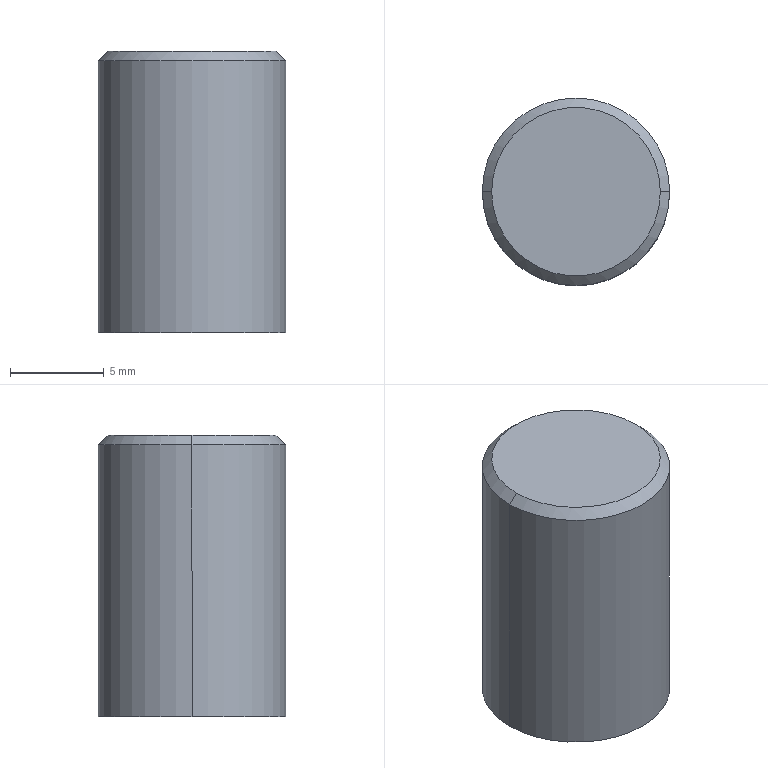Part | SolidWorks | features BaseBody 1 | 1 solid | 6 faces | box 10 x 10 x 15 mm | volume 1174 mm3 | cone 2 | cylinder 2 | plane 2 | commonest cylinder face diameters 10 x2
STEP:
#1=CARTESIAN_POINT('',(-4.5,0.,15.));
#2=VERTEX_POINT('',#1);
#3=CARTESIAN_POINT('',(4.5,0.,15.));
#4=VERTEX_POINT('',#3);
#5=CARTESIAN_POINT('',(0.,0.,15.));
#6=DIRECTION('',(0.,0.,-1.));
#7=DIRECTION('',(-1.,0.,0.));
#8=AXIS2_PLACEMENT_3D('',#5,#6,#7);
#9=CIRCLE('',#8,4.5);
#10=EDGE_CURVE('',#2,#4,#9,.T.);
#11=ORIENTED_EDGE('',*,*,#10,.T.);
#12=CARTESIAN_POINT('',(5.,0.,14.5));
#13=VERTEX_POINT('',#12);
#14=CARTESIAN_POINT('',(4.75,0.,14.75));
#15=DIRECTION('',(0.7071,0.,-0.7071));
#16=VECTOR('',#15,1000.);
#17=LINE('',#14,#16);
#18=EDGE_CURVE('',#4,#13,#17,.T.);
#19=ORIENTED_EDGE('',*,*,#18,.T.);
#20=CARTESIAN_POINT('',(-5.,0.,14.5));
#21=VERTEX_POINT('',#20);
#22=CARTESIAN_POINT('',(0.,0.,14.5));
#23=DIRECTION('',(0.,0.,1.));
#24=DIRECTION('',(-1.,0.,0.));
#25=AXIS2_PLACEMENT_3D('',#22,#23,#24);
#26=CIRCLE('',#25,5.);
#27=EDGE_CURVE('',#13,#21,#26,.T.);
#28=ORIENTED_EDGE('',*,*,#27,.T.);
#29=CARTESIAN_POINT('',(-4.75,0.,14.75));
#30=DIRECTION('',(-0.7071,0.,-0.7071));
#31=VECTOR('',#30,1000.);
#32=LINE('',#29,#31);
#33=EDGE_CURVE('',#2,#21,#32,.T.);
#34=ORIENTED_EDGE('',*,*,#33,.F.);
#35=EDGE_LOOP('',(#11,#19,#28,#34));
#36=FACE_OUTER_BOUND('',#35,.T.);
#37=CARTESIAN_POINT('',(0.,0.,14.75));
#38=DIRECTION('',(0.,0.,-1.));
#39=DIRECTION('',(-1.,0.,0.));
#40=AXIS2_PLACEMENT_3D('',#37,#38,#39);
#41=CONICAL_SURFACE('',#40,4.75,0.7854);
#42=ADVANCED_FACE('',(#36),#41,.T.);
#43=CARTESIAN_POINT('',(5.,0.,0.));
#44=VERTEX_POINT('',#43);
#45=CARTESIAN_POINT('',(-5.,0.,0.));
#46=VERTEX_POINT('',#45);
#47=CARTESIAN_POINT('',(0.,0.,0.));
#48=DIRECTION('',(0.,0.,-1.));
#49=DIRECTION('',(-1.,0.,0.));
#50=AXIS2_PLACEMENT_3D('',#47,#48,#49);
#51=CIRCLE('',#50,5.);
#52=EDGE_CURVE('',#44,#46,#51,.T.);
#53=ORIENTED_EDGE('',*,*,#52,.F.);
#54=CARTESIAN_POINT('',(5.,0.,0.));
#55=DIRECTION('',(0.,0.,1.));
#56=VECTOR('',#55,1000.);
#57=LINE('',#54,#56);
#58=EDGE_CURVE('',#44,#13,#57,.T.);
#59=ORIENTED_EDGE('',*,*,#58,.T.);
#60=CARTESIAN_POINT('',(0.,0.,14.5));
#61=DIRECTION('',(0.,0.,1.));
#62=DIRECTION('',(-1.,0.,0.));
#63=AXIS2_PLACEMENT_3D('',#60,#61,#62);
#64=CIRCLE('',#63,5.);
#65=EDGE_CURVE('',#21,#13,#64,.T.);
#66=ORIENTED_EDGE('',*,*,#65,.F.);
#67=CARTESIAN_POINT('',(-5.,0.,0.));
#68=DIRECTION('',(0.,0.,1.));
#69=VECTOR('',#68,1000.);
#70=LINE('',#67,#69);
#71=EDGE_CURVE('',#46,#21,#70,.T.);
#72=ORIENTED_EDGE('',*,*,#71,.F.);
#73=EDGE_LOOP('',(#53,#59,#66,#72));
#74=FACE_OUTER_BOUND('',#73,.T.);
#75=CARTESIAN_POINT('',(0.,0.,0.));
#76=DIRECTION('',(0.,0.,1.));
#77=DIRECTION('',(-1.,0.,0.));
#78=AXIS2_PLACEMENT_3D('',#75,#76,#77);
#79=CYLINDRICAL_SURFACE('',#78,5.);
#80=ADVANCED_FACE('',(#74),#79,.T.);
#81=CARTESIAN_POINT('',(0.,0.,0.));
#82=DIRECTION('',(0.,0.,-1.));
#83=DIRECTION('',(-1.,0.,0.));
#84=AXIS2_PLACEMENT_3D('',#81,#82,#83);
#85=CIRCLE('',#84,5.);
#86=EDGE_CURVE('',#46,#44,#85,.T.);
#87=ORIENTED_EDGE('',*,*,#86,.T.);
#88=ORIENTED_EDGE('',*,*,#52,.T.);
#89=EDGE_LOOP('',(#87,#88));
#90=FACE_OUTER_BOUND('',#89,.T.);
#91=CARTESIAN_POINT('',(0.,0.,0.));
#92=DIRECTION('',(0.,0.,1.));
#93=DIRECTION('',(1.,0.,0.));
#94=AXIS2_PLACEMENT_3D('',#91,#92,#93);
#95=PLANE('',#94);
#96=ADVANCED_FACE('',(#90),#95,.F.);
#97=ORIENTED_EDGE('',*,*,#10,.F.);
#98=CARTESIAN_POINT('',(0.,0.,15.));
#99=DIRECTION('',(0.,0.,-1.));
#100=DIRECTION('',(-1.,0.,0.));
#101=AXIS2_PLACEMENT_3D('',#98,#99,#100);
#102=CIRCLE('',#101,4.5);
#103=EDGE_CURVE('',#4,#2,#102,.T.);
#104=ORIENTED_EDGE('',*,*,#103,.F.);
#105=EDGE_LOOP('',(#97,#104));
#106=FACE_OUTER_BOUND('',#105,.T.);
#107=CARTESIAN_POINT('',(0.,0.,15.));
#108=DIRECTION('',(0.,0.,1.));
#109=DIRECTION('',(1.,0.,0.));
#110=AXIS2_PLACEMENT_3D('',#107,#108,#109);
#111=PLANE('',#110);
#112=ADVANCED_FACE('',(#106),#111,.T.);
#113=ORIENTED_EDGE('',*,*,#58,.F.);
#114=ORIENTED_EDGE('',*,*,#86,.F.);
#115=ORIENTED_EDGE('',*,*,#71,.T.);
#116=ORIENTED_EDGE('',*,*,#27,.F.);
#117=EDGE_LOOP('',(#113,#114,#115,#116));
#118=FACE_OUTER_BOUND('',#117,.T.);
#119=CARTESIAN_POINT('',(0.,0.,0.));
#120=DIRECTION('',(0.,0.,1.));
#121=DIRECTION('',(-1.,0.,0.));
#122=AXIS2_PLACEMENT_3D('',#119,#120,#121);
#123=CYLINDRICAL_SURFACE('',#122,5.);
#124=ADVANCED_FACE('',(#118),#123,.T.);
#125=ORIENTED_EDGE('',*,*,#18,.F.);
#126=ORIENTED_EDGE('',*,*,#103,.T.);
#127=ORIENTED_EDGE('',*,*,#33,.T.);
#128=ORIENTED_EDGE('',*,*,#65,.T.);
#129=EDGE_LOOP('',(#125,#126,#127,#128));
#130=FACE_OUTER_BOUND('',#129,.T.);
#131=CARTESIAN_POINT('',(0.,0.,14.75));
#132=DIRECTION('',(0.,0.,-1.));
#133=DIRECTION('',(-1.,0.,0.));
#134=AXIS2_PLACEMENT_3D('',#131,#132,#133);
#135=CONICAL_SURFACE('',#134,4.75,0.7854);
#136=ADVANCED_FACE('',(#130),#135,.T.);
#137=CLOSED_SHELL('',(#42,#80,#96,#112,#124,#136));
#138=MANIFOLD_SOLID_BREP('',#137);
#139=CARTESIAN_POINT('',(0.,0.,0.));
#140=DIRECTION('',(0.,0.,1.));
#141=DIRECTION('',(1.,0.,0.));
#142=AXIS2_PLACEMENT_3D('',#139,#140,#141);
#143=(LENGTH_UNIT()NAMED_UNIT(*)SI_UNIT(.MILLI.,.METRE.));
#144=UNCERTAINTY_MEASURE_WITH_UNIT(LENGTH_MEASURE(0.00001),#143,'','');
#145=(NAMED_UNIT(*)PLANE_ANGLE_UNIT()SI_UNIT($,.RADIAN.));
#146=(NAMED_UNIT(*)SI_UNIT($,.STERADIAN.)SOLID_ANGLE_UNIT());
#147=(GEOMETRIC_REPRESENTATION_CONTEXT(3)GLOBAL_UNCERTAINTY_ASSIGNED_CONTEXT((#144))GLOBAL_UNIT_ASSIGNED_CONTEXT((#143,#145,#146))REPRESENTATION_CONTEXT('',''));
#148=ADVANCED_BREP_SHAPE_REPRESENTATION('',(#138,#142),#147);